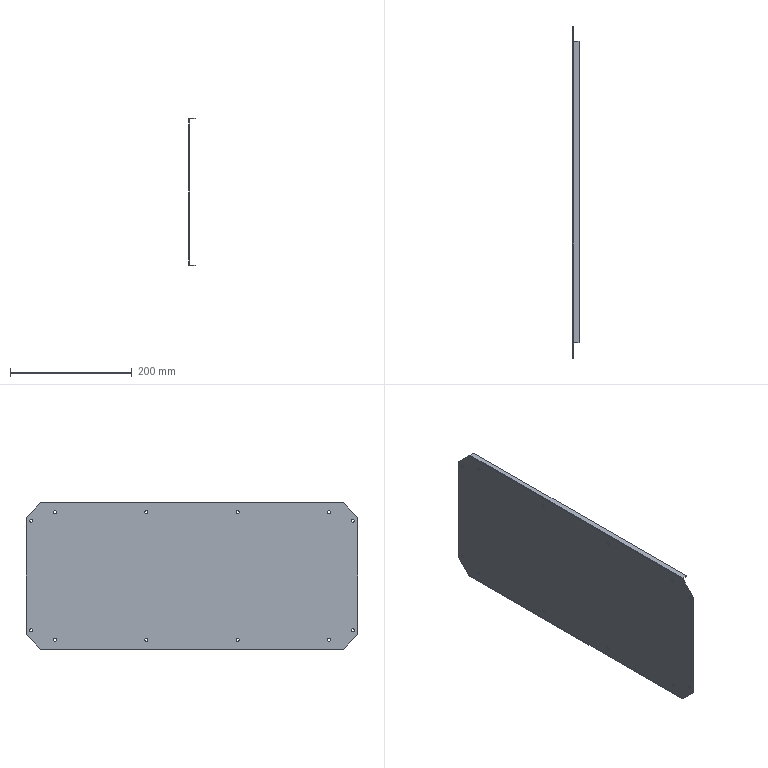Part | STEP file | RJWD-DY-0102_X2_5DE667DC95E8_39 | 1 solid | 50 faces | box 10 x 545 x 243 mm | volume 139493 mm3 | cylinder 28 | plane 18 | spline 4 | commonest cylinder face diameters 5 x24 0.4 x2 2.4 x2